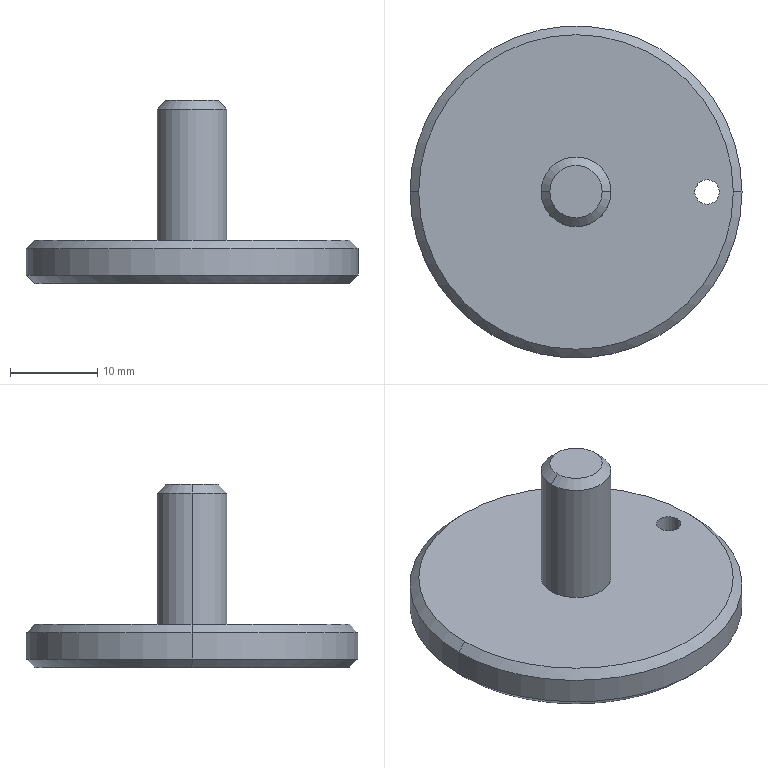Part | STEP file | Pulley locating pin | 1 solid | 15 faces | box 38 x 38 x 21 mm | volume 6315 mm3 | cylinder 6 | cone 6 | plane 3 | commonest cylinder face diameters 2.8 x2 8 x2 38 x2
STEP:
#1=CARTESIAN_POINT('',(13.6,0.,0.));
#2=VERTEX_POINT('',#1);
#3=CARTESIAN_POINT('',(16.4,0.,0.));
#4=VERTEX_POINT('',#3);
#5=CARTESIAN_POINT('',(15.,0.,0.));
#6=DIRECTION('',(0.,0.,1.));
#7=DIRECTION('',(1.,0.,0.));
#8=AXIS2_PLACEMENT_3D('',#5,#6,#7);
#9=CIRCLE('',#8,1.4);
#10=EDGE_CURVE('',#2,#4,#9,.T.);
#11=ORIENTED_EDGE('',*,*,#10,.F.);
#12=CARTESIAN_POINT('',(13.6,0.,5.));
#13=VERTEX_POINT('',#12);
#14=CARTESIAN_POINT('',(13.6,0.,-5.));
#15=DIRECTION('',(0.,0.,1.));
#16=VECTOR('',#15,1000.);
#17=LINE('',#14,#16);
#18=EDGE_CURVE('',#2,#13,#17,.T.);
#19=ORIENTED_EDGE('',*,*,#18,.T.);
#20=CARTESIAN_POINT('',(16.4,0.,5.));
#21=VERTEX_POINT('',#20);
#22=CARTESIAN_POINT('',(15.,0.,5.));
#23=DIRECTION('',(0.,0.,1.));
#24=DIRECTION('',(1.,0.,0.));
#25=AXIS2_PLACEMENT_3D('',#22,#23,#24);
#26=CIRCLE('',#25,1.4);
#27=EDGE_CURVE('',#13,#21,#26,.T.);
#28=ORIENTED_EDGE('',*,*,#27,.T.);
#29=CARTESIAN_POINT('',(16.4,0.,-5.));
#30=DIRECTION('',(0.,0.,1.));
#31=VECTOR('',#30,1000.);
#32=LINE('',#29,#31);
#33=EDGE_CURVE('',#4,#21,#32,.T.);
#34=ORIENTED_EDGE('',*,*,#33,.F.);
#35=EDGE_LOOP('',(#11,#19,#28,#34));
#36=FACE_OUTER_BOUND('',#35,.T.);
#37=CARTESIAN_POINT('',(15.,0.,-5.));
#38=DIRECTION('',(0.,0.,1.));
#39=DIRECTION('',(1.,0.,0.));
#40=AXIS2_PLACEMENT_3D('',#37,#38,#39);
#41=CYLINDRICAL_SURFACE('',#40,1.4);
#42=ADVANCED_FACE('',(#36),#41,.F.);
#43=CARTESIAN_POINT('',(-18.,0.,0.));
#44=VERTEX_POINT('',#43);
#45=CARTESIAN_POINT('',(18.,0.,0.));
#46=VERTEX_POINT('',#45);
#47=CARTESIAN_POINT('',(0.,0.,0.));
#48=DIRECTION('',(0.,0.,-1.));
#49=DIRECTION('',(1.,0.,0.));
#50=AXIS2_PLACEMENT_3D('',#47,#48,#49);
#51=CIRCLE('',#50,18.);
#52=EDGE_CURVE('',#44,#46,#51,.T.);
#53=ORIENTED_EDGE('',*,*,#52,.F.);
#54=CARTESIAN_POINT('',(-19.,0.,1.));
#55=VERTEX_POINT('',#54);
#56=CARTESIAN_POINT('',(-19.,0.,1.));
#57=DIRECTION('',(-0.7071,0.,0.7071));
#58=VECTOR('',#57,1000.);
#59=LINE('',#56,#58);
#60=EDGE_CURVE('',#44,#55,#59,.T.);
#61=ORIENTED_EDGE('',*,*,#60,.T.);
#62=CARTESIAN_POINT('',(19.,0.,1.));
#63=VERTEX_POINT('',#62);
#64=CARTESIAN_POINT('',(0.,0.,1.));
#65=DIRECTION('',(0.,0.,1.));
#66=DIRECTION('',(1.,0.,0.));
#67=AXIS2_PLACEMENT_3D('',#64,#65,#66);
#68=CIRCLE('',#67,19.);
#69=EDGE_CURVE('',#63,#55,#68,.T.);
#70=ORIENTED_EDGE('',*,*,#69,.F.);
#71=CARTESIAN_POINT('',(19.,0.,1.));
#72=DIRECTION('',(0.7071,0.,0.7071));
#73=VECTOR('',#72,1000.);
#74=LINE('',#71,#73);
#75=EDGE_CURVE('',#46,#63,#74,.T.);
#76=ORIENTED_EDGE('',*,*,#75,.F.);
#77=EDGE_LOOP('',(#53,#61,#70,#76));
#78=FACE_OUTER_BOUND('',#77,.T.);
#79=CARTESIAN_POINT('',(0.,0.,1.));
#80=DIRECTION('',(0.,0.,1.));
#81=DIRECTION('',(1.,0.,0.));
#82=AXIS2_PLACEMENT_3D('',#79,#80,#81);
#83=CONICAL_SURFACE('',#82,19.,0.7854);
#84=ADVANCED_FACE('',(#78),#83,.T.);
#85=CARTESIAN_POINT('',(18.,0.,5.));
#86=VERTEX_POINT('',#85);
#87=CARTESIAN_POINT('',(-18.,0.,5.));
#88=VERTEX_POINT('',#87);
#89=CARTESIAN_POINT('',(0.,0.,5.));
#90=DIRECTION('',(0.,0.,1.));
#91=DIRECTION('',(1.,0.,0.));
#92=AXIS2_PLACEMENT_3D('',#89,#90,#91);
#93=CIRCLE('',#92,18.);
#94=EDGE_CURVE('',#86,#88,#93,.T.);
#95=ORIENTED_EDGE('',*,*,#94,.F.);
#96=CARTESIAN_POINT('',(19.,0.,4.));
#97=VERTEX_POINT('',#96);
#98=CARTESIAN_POINT('',(18.,0.,5.));
#99=DIRECTION('',(0.7071,0.,-0.7071));
#100=VECTOR('',#99,1000.);
#101=LINE('',#98,#100);
#102=EDGE_CURVE('',#86,#97,#101,.T.);
#103=ORIENTED_EDGE('',*,*,#102,.T.);
#104=CARTESIAN_POINT('',(-19.,0.,4.));
#105=VERTEX_POINT('',#104);
#106=CARTESIAN_POINT('',(0.,0.,4.));
#107=DIRECTION('',(0.,0.,-1.));
#108=DIRECTION('',(1.,0.,0.));
#109=AXIS2_PLACEMENT_3D('',#106,#107,#108);
#110=CIRCLE('',#109,19.);
#111=EDGE_CURVE('',#105,#97,#110,.T.);
#112=ORIENTED_EDGE('',*,*,#111,.F.);
#113=CARTESIAN_POINT('',(-18.,0.,5.));
#114=DIRECTION('',(-0.7071,0.,-0.7071));
#115=VECTOR('',#114,1000.);
#116=LINE('',#113,#115);
#117=EDGE_CURVE('',#88,#105,#116,.T.);
#118=ORIENTED_EDGE('',*,*,#117,.F.);
#119=EDGE_LOOP('',(#95,#103,#112,#118));
#120=FACE_OUTER_BOUND('',#119,.T.);
#121=CARTESIAN_POINT('',(0.,0.,5.));
#122=DIRECTION('',(0.,0.,-1.));
#123=DIRECTION('',(-1.,0.,0.));
#124=AXIS2_PLACEMENT_3D('',#121,#122,#123);
#125=CONICAL_SURFACE('',#124,18.,0.7854);
#126=ADVANCED_FACE('',(#120),#125,.T.);
#127=CARTESIAN_POINT('',(3.,0.,21.));
#128=VERTEX_POINT('',#127);
#129=CARTESIAN_POINT('',(-3.,0.,21.));
#130=VERTEX_POINT('',#129);
#131=CARTESIAN_POINT('',(0.,0.,21.));
#132=DIRECTION('',(0.,0.,1.));
#133=DIRECTION('',(1.,0.,0.));
#134=AXIS2_PLACEMENT_3D('',#131,#132,#133);
#135=CIRCLE('',#134,3.);
#136=EDGE_CURVE('',#128,#130,#135,.T.);
#137=ORIENTED_EDGE('',*,*,#136,.F.);
#138=CARTESIAN_POINT('',(4.,0.,20.));
#139=VERTEX_POINT('',#138);
#140=CARTESIAN_POINT('',(3.,0.,21.));
#141=DIRECTION('',(0.7071,0.,-0.7071));
#142=VECTOR('',#141,1000.);
#143=LINE('',#140,#142);
#144=EDGE_CURVE('',#128,#139,#143,.T.);
#145=ORIENTED_EDGE('',*,*,#144,.T.);
#146=CARTESIAN_POINT('',(-4.,0.,20.));
#147=VERTEX_POINT('',#146);
#148=CARTESIAN_POINT('',(0.,0.,20.));
#149=DIRECTION('',(0.,0.,-1.));
#150=DIRECTION('',(1.,0.,0.));
#151=AXIS2_PLACEMENT_3D('',#148,#149,#150);
#152=CIRCLE('',#151,4.);
#153=EDGE_CURVE('',#147,#139,#152,.T.);
#154=ORIENTED_EDGE('',*,*,#153,.F.);
#155=CARTESIAN_POINT('',(-3.,0.,21.));
#156=DIRECTION('',(-0.7071,0.,-0.7071));
#157=VECTOR('',#156,1000.);
#158=LINE('',#155,#157);
#159=EDGE_CURVE('',#130,#147,#158,.T.);
#160=ORIENTED_EDGE('',*,*,#159,.F.);
#161=EDGE_LOOP('',(#137,#145,#154,#160));
#162=FACE_OUTER_BOUND('',#161,.T.);
#163=CARTESIAN_POINT('',(0.,0.,21.));
#164=DIRECTION('',(0.,0.,-1.));
#165=DIRECTION('',(-1.,0.,0.));
#166=AXIS2_PLACEMENT_3D('',#163,#164,#165);
#167=CONICAL_SURFACE('',#166,3.,0.7854);
#168=ADVANCED_FACE('',(#162),#167,.T.);
#169=ORIENTED_EDGE('',*,*,#153,.T.);
#170=CARTESIAN_POINT('',(4.,0.,5.));
#171=VERTEX_POINT('',#170);
#172=CARTESIAN_POINT('',(4.,0.,21.));
#173=DIRECTION('',(0.,0.,-1.));
#174=VECTOR('',#173,1000.);
#175=LINE('',#172,#174);
#176=EDGE_CURVE('',#139,#171,#175,.T.);
#177=ORIENTED_EDGE('',*,*,#176,.T.);
#178=CARTESIAN_POINT('',(-4.,0.,5.));
#179=VERTEX_POINT('',#178);
#180=CARTESIAN_POINT('',(0.,0.,5.));
#181=DIRECTION('',(0.,0.,1.));
#182=DIRECTION('',(1.,0.,0.));
#183=AXIS2_PLACEMENT_3D('',#180,#181,#182);
#184=CIRCLE('',#183,4.);
#185=EDGE_CURVE('',#171,#179,#184,.T.);
#186=ORIENTED_EDGE('',*,*,#185,.T.);
#187=CARTESIAN_POINT('',(-4.,0.,21.));
#188=DIRECTION('',(0.,0.,-1.));
#189=VECTOR('',#188,1000.);
#190=LINE('',#187,#189);
#191=EDGE_CURVE('',#147,#179,#190,.T.);
#192=ORIENTED_EDGE('',*,*,#191,.F.);
#193=EDGE_LOOP('',(#169,#177,#186,#192));
#194=FACE_OUTER_BOUND('',#193,.T.);
#195=CARTESIAN_POINT('',(0.,0.,21.));
#196=DIRECTION('',(0.,0.,-1.));
#197=DIRECTION('',(-1.,0.,0.));
#198=AXIS2_PLACEMENT_3D('',#195,#196,#197);
#199=CYLINDRICAL_SURFACE('',#198,4.);
#200=ADVANCED_FACE('',(#194),#199,.T.);
#201=ORIENTED_EDGE('',*,*,#111,.T.);
#202=CARTESIAN_POINT('',(19.,0.,5.));
#203=DIRECTION('',(0.,0.,-1.));
#204=VECTOR('',#203,1000.);
#205=LINE('',#202,#204);
#206=EDGE_CURVE('',#97,#63,#205,.T.);
#207=ORIENTED_EDGE('',*,*,#206,.T.);
#208=ORIENTED_EDGE('',*,*,#69,.T.);
#209=CARTESIAN_POINT('',(-19.,0.,5.));
#210=DIRECTION('',(0.,0.,-1.));
#211=VECTOR('',#210,1000.);
#212=LINE('',#209,#211);
#213=EDGE_CURVE('',#105,#55,#212,.T.);
#214=ORIENTED_EDGE('',*,*,#213,.F.);
#215=EDGE_LOOP('',(#201,#207,#208,#214));
#216=FACE_OUTER_BOUND('',#215,.T.);
#217=CARTESIAN_POINT('',(0.,0.,5.));
#218=DIRECTION('',(0.,0.,-1.));
#219=DIRECTION('',(-1.,0.,0.));
#220=AXIS2_PLACEMENT_3D('',#217,#218,#219);
#221=CYLINDRICAL_SURFACE('',#220,19.);
#222=ADVANCED_FACE('',(#216),#221,.T.);
#223=ORIENTED_EDGE('',*,*,#206,.F.);
#224=CARTESIAN_POINT('',(0.,0.,4.));
#225=DIRECTION('',(0.,0.,-1.));
#226=DIRECTION('',(1.,0.,0.));
#227=AXIS2_PLACEMENT_3D('',#224,#225,#226);
#228=CIRCLE('',#227,19.);
#229=EDGE_CURVE('',#97,#105,#228,.T.);
#230=ORIENTED_EDGE('',*,*,#229,.T.);
#231=ORIENTED_EDGE('',*,*,#213,.T.);
#232=CARTESIAN_POINT('',(0.,0.,1.));
#233=DIRECTION('',(0.,0.,1.));
#234=DIRECTION('',(1.,0.,0.));
#235=AXIS2_PLACEMENT_3D('',#232,#233,#234);
#236=CIRCLE('',#235,19.);
#237=EDGE_CURVE('',#55,#63,#236,.T.);
#238=ORIENTED_EDGE('',*,*,#237,.T.);
#239=EDGE_LOOP('',(#223,#230,#231,#238));
#240=FACE_OUTER_BOUND('',#239,.T.);
#241=CARTESIAN_POINT('',(0.,0.,5.));
#242=DIRECTION('',(0.,0.,-1.));
#243=DIRECTION('',(-1.,0.,0.));
#244=AXIS2_PLACEMENT_3D('',#241,#242,#243);
#245=CYLINDRICAL_SURFACE('',#244,19.);
#246=ADVANCED_FACE('',(#240),#245,.T.);
#247=CARTESIAN_POINT('',(15.,0.,5.));
#248=DIRECTION('',(0.,0.,1.));
#249=DIRECTION('',(1.,0.,0.));
#250=AXIS2_PLACEMENT_3D('',#247,#248,#249);
#251=CIRCLE('',#250,1.4);
#252=EDGE_CURVE('',#21,#13,#251,.T.);
#253=ORIENTED_EDGE('',*,*,#252,.F.);
#254=ORIENTED_EDGE('',*,*,#27,.F.);
#255=EDGE_LOOP('',(#253,#254));
#256=FACE_BOUND('',#255,.T.);
#257=CARTESIAN_POINT('',(0.,0.,5.));
#258=DIRECTION('',(0.,0.,1.));
#259=DIRECTION('',(1.,0.,0.));
#260=AXIS2_PLACEMENT_3D('',#257,#258,#259);
#261=CIRCLE('',#260,18.);
#262=EDGE_CURVE('',#88,#86,#261,.T.);
#263=ORIENTED_EDGE('',*,*,#262,.T.);
#264=ORIENTED_EDGE('',*,*,#94,.T.);
#265=EDGE_LOOP('',(#263,#264));
#266=FACE_OUTER_BOUND('',#265,.T.);
#267=CARTESIAN_POINT('',(0.,0.,5.));
#268=DIRECTION('',(0.,0.,1.));
#269=DIRECTION('',(1.,0.,0.));
#270=AXIS2_PLACEMENT_3D('',#267,#268,#269);
#271=CIRCLE('',#270,4.);
#272=EDGE_CURVE('',#179,#171,#271,.T.);
#273=ORIENTED_EDGE('',*,*,#272,.F.);
#274=ORIENTED_EDGE('',*,*,#185,.F.);
#275=EDGE_LOOP('',(#273,#274));
#276=FACE_BOUND('',#275,.T.);
#277=CARTESIAN_POINT('',(0.,0.,5.));
#278=DIRECTION('',(0.,0.,1.));
#279=DIRECTION('',(1.,0.,0.));
#280=AXIS2_PLACEMENT_3D('',#277,#278,#279);
#281=PLANE('',#280);
#282=ADVANCED_FACE('',(#256,#266,#276),#281,.T.);
#283=CARTESIAN_POINT('',(15.,0.,0.));
#284=DIRECTION('',(0.,0.,1.));
#285=DIRECTION('',(1.,0.,0.));
#286=AXIS2_PLACEMENT_3D('',#283,#284,#285);
#287=CIRCLE('',#286,1.4);
#288=EDGE_CURVE('',#4,#2,#287,.T.);
#289=ORIENTED_EDGE('',*,*,#288,.T.);
#290=ORIENTED_EDGE('',*,*,#10,.T.);
#291=EDGE_LOOP('',(#289,#290));
#292=FACE_BOUND('',#291,.T.);
#293=CARTESIAN_POINT('',(0.,0.,0.));
#294=DIRECTION('',(0.,0.,-1.));
#295=DIRECTION('',(1.,0.,0.));
#296=AXIS2_PLACEMENT_3D('',#293,#294,#295);
#297=CIRCLE('',#296,18.);
#298=EDGE_CURVE('',#46,#44,#297,.T.);
#299=ORIENTED_EDGE('',*,*,#298,.T.);
#300=ORIENTED_EDGE('',*,*,#52,.T.);
#301=EDGE_LOOP('',(#299,#300));
#302=FACE_OUTER_BOUND('',#301,.T.);
#303=CARTESIAN_POINT('',(0.,0.,0.));
#304=DIRECTION('',(0.,0.,1.));
#305=DIRECTION('',(1.,0.,0.));
#306=AXIS2_PLACEMENT_3D('',#303,#304,#305);
#307=PLANE('',#306);
#308=ADVANCED_FACE('',(#292,#302),#307,.F.);
#309=ORIENTED_EDGE('',*,*,#176,.F.);
#310=CARTESIAN_POINT('',(0.,0.,20.));
#311=DIRECTION('',(0.,0.,-1.));
#312=DIRECTION('',(1.,0.,0.));
#313=AXIS2_PLACEMENT_3D('',#310,#311,#312);
#314=CIRCLE('',#313,4.);
#315=EDGE_CURVE('',#139,#147,#314,.T.);
#316=ORIENTED_EDGE('',*,*,#315,.T.);
#317=ORIENTED_EDGE('',*,*,#191,.T.);
#318=ORIENTED_EDGE('',*,*,#272,.T.);
#319=EDGE_LOOP('',(#309,#316,#317,#318));
#320=FACE_OUTER_BOUND('',#319,.T.);
#321=CARTESIAN_POINT('',(0.,0.,21.));
#322=DIRECTION('',(0.,0.,-1.));
#323=DIRECTION('',(-1.,0.,0.));
#324=AXIS2_PLACEMENT_3D('',#321,#322,#323);
#325=CYLINDRICAL_SURFACE('',#324,4.);
#326=ADVANCED_FACE('',(#320),#325,.T.);
#327=CARTESIAN_POINT('',(0.,0.,21.));
#328=DIRECTION('',(0.,0.,1.));
#329=DIRECTION('',(1.,0.,0.));
#330=AXIS2_PLACEMENT_3D('',#327,#328,#329);
#331=CIRCLE('',#330,3.);
#332=EDGE_CURVE('',#130,#128,#331,.T.);
#333=ORIENTED_EDGE('',*,*,#332,.T.);
#334=ORIENTED_EDGE('',*,*,#136,.T.);
#335=EDGE_LOOP('',(#333,#334));
#336=FACE_OUTER_BOUND('',#335,.T.);
#337=CARTESIAN_POINT('',(0.,0.,21.));
#338=DIRECTION('',(0.,0.,1.));
#339=DIRECTION('',(1.,0.,0.));
#340=AXIS2_PLACEMENT_3D('',#337,#338,#339);
#341=PLANE('',#340);
#342=ADVANCED_FACE('',(#336),#341,.T.);
#343=ORIENTED_EDGE('',*,*,#144,.F.);
#344=ORIENTED_EDGE('',*,*,#332,.F.);
#345=ORIENTED_EDGE('',*,*,#159,.T.);
#346=ORIENTED_EDGE('',*,*,#315,.F.);
#347=EDGE_LOOP('',(#343,#344,#345,#346));
#348=FACE_OUTER_BOUND('',#347,.T.);
#349=CARTESIAN_POINT('',(0.,0.,21.));
#350=DIRECTION('',(0.,0.,-1.));
#351=DIRECTION('',(-1.,0.,0.));
#352=AXIS2_PLACEMENT_3D('',#349,#350,#351);
#353=CONICAL_SURFACE('',#352,3.,0.7854);
#354=ADVANCED_FACE('',(#348),#353,.T.);
#355=ORIENTED_EDGE('',*,*,#102,.F.);
#356=ORIENTED_EDGE('',*,*,#262,.F.);
#357=ORIENTED_EDGE('',*,*,#117,.T.);
#358=ORIENTED_EDGE('',*,*,#229,.F.);
#359=EDGE_LOOP('',(#355,#356,#357,#358));
#360=FACE_OUTER_BOUND('',#359,.T.);
#361=CARTESIAN_POINT('',(0.,0.,5.));
#362=DIRECTION('',(0.,0.,-1.));
#363=DIRECTION('',(-1.,0.,0.));
#364=AXIS2_PLACEMENT_3D('',#361,#362,#363);
#365=CONICAL_SURFACE('',#364,18.,0.7854);
#366=ADVANCED_FACE('',(#360),#365,.T.);
#367=ORIENTED_EDGE('',*,*,#60,.F.);
#368=ORIENTED_EDGE('',*,*,#298,.F.);
#369=ORIENTED_EDGE('',*,*,#75,.T.);
#370=ORIENTED_EDGE('',*,*,#237,.F.);
#371=EDGE_LOOP('',(#367,#368,#369,#370));
#372=FACE_OUTER_BOUND('',#371,.T.);
#373=CARTESIAN_POINT('',(0.,0.,1.));
#374=DIRECTION('',(0.,0.,1.));
#375=DIRECTION('',(1.,0.,0.));
#376=AXIS2_PLACEMENT_3D('',#373,#374,#375);
#377=CONICAL_SURFACE('',#376,19.,0.7854);
#378=ADVANCED_FACE('',(#372),#377,.T.);
#379=ORIENTED_EDGE('',*,*,#18,.F.);
#380=ORIENTED_EDGE('',*,*,#288,.F.);
#381=ORIENTED_EDGE('',*,*,#33,.T.);
#382=ORIENTED_EDGE('',*,*,#252,.T.);
#383=EDGE_LOOP('',(#379,#380,#381,#382));
#384=FACE_OUTER_BOUND('',#383,.T.);
#385=CARTESIAN_POINT('',(15.,0.,-5.));
#386=DIRECTION('',(0.,0.,1.));
#387=DIRECTION('',(1.,0.,0.));
#388=AXIS2_PLACEMENT_3D('',#385,#386,#387);
#389=CYLINDRICAL_SURFACE('',#388,1.4);
#390=ADVANCED_FACE('',(#384),#389,.F.);
#391=CLOSED_SHELL('',(#42,#84,#126,#168,#200,#222,#246,#282,#308,#326,#342,#354,#366,#378,#390));
#392=MANIFOLD_SOLID_BREP('',#391);
#393=CARTESIAN_POINT('',(0.,0.,0.));
#394=DIRECTION('',(0.,0.,1.));
#395=DIRECTION('',(1.,0.,0.));
#396=AXIS2_PLACEMENT_3D('',#393,#394,#395);
#397=(LENGTH_UNIT()NAMED_UNIT(*)SI_UNIT(.MILLI.,.METRE.));
#398=UNCERTAINTY_MEASURE_WITH_UNIT(LENGTH_MEASURE(0.00001),#397,'','');
#399=(NAMED_UNIT(*)PLANE_ANGLE_UNIT()SI_UNIT($,.RADIAN.));
#400=(NAMED_UNIT(*)SI_UNIT($,.STERADIAN.)SOLID_ANGLE_UNIT());
#401=(GEOMETRIC_REPRESENTATION_CONTEXT(3)GLOBAL_UNCERTAINTY_ASSIGNED_CONTEXT((#398))GLOBAL_UNIT_ASSIGNED_CONTEXT((#397,#399,#400))REPRESENTATION_CONTEXT('',''));
#402=ADVANCED_BREP_SHAPE_REPRESENTATION('',(#392,#396),#401);